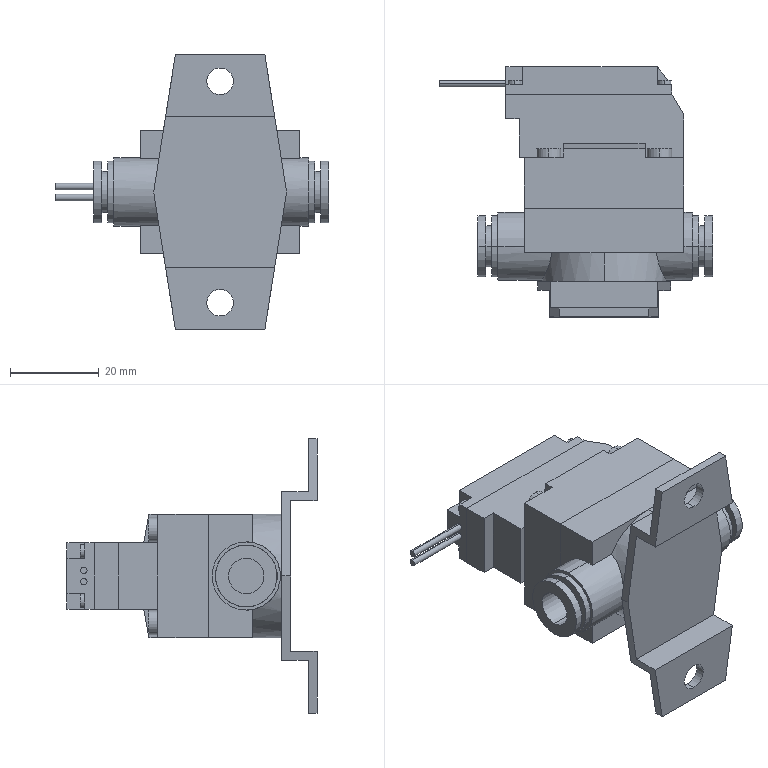Part | STEP file | EXA-C8-02CB-3(1) blow-off valve | 4 solids | 140 faces | box 61.7 x 56.5 x 62 mm | volume 42918 mm3 | plane 90 | cylinder 50 | commonest cylinder face diameters 3 x8 5.5 x8 1.5 x4 2.6 x4 6 x4 8 x4